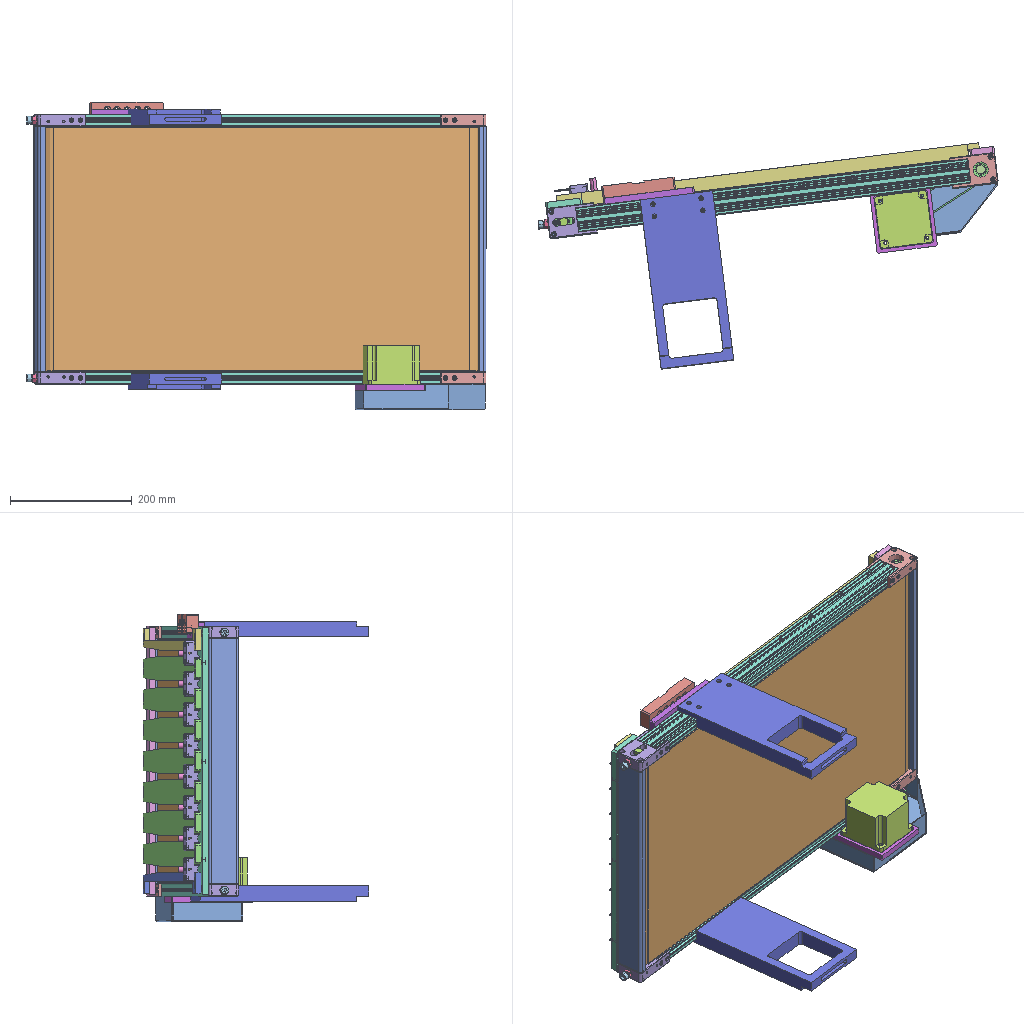Assembly | STEP file | 35 different items | 337 placed | box 756 x 372 x 506 mm
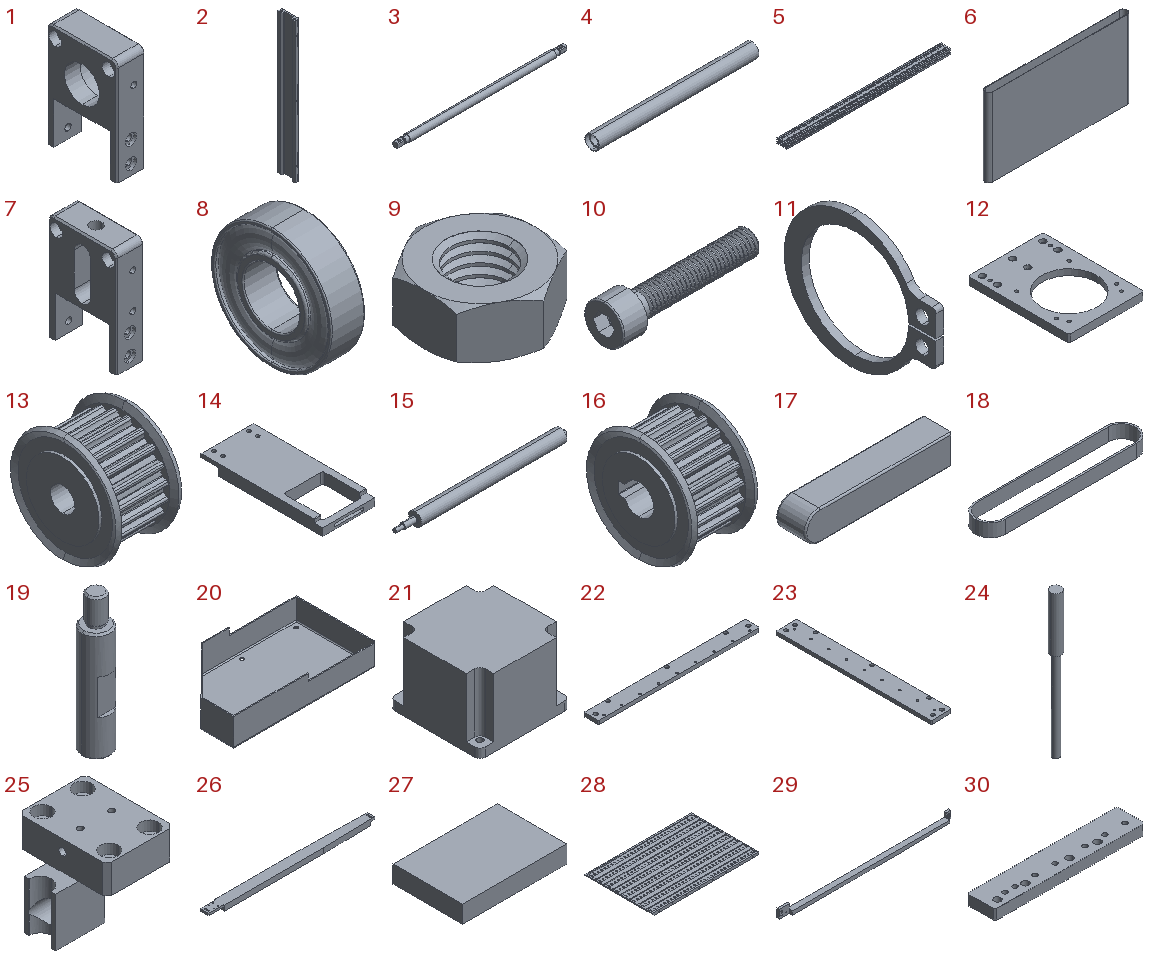Parts list (item | name | quantity | parent item | size | volume):
1 | PN_0002 | x2 | in 30 | 20 x 50 x 75 mm | 35811 mm3
2 | PN_0016 | x2 | in 30 | 12 x 50 x 404 mm | 142558 mm3
3 | PN_0017 | x1 | in 30 | 444 x 18 x 18 mm | 106069 mm3
4 | PN_0018 | x1 | in 30 | 402 x 36 x 36 mm | 206186 mm3
5 | PN_0005_default[machined] | x2 | in 30 | 650 x 40 x 20 mm | 192154 mm3
6 | PN_0019 | x1 | in 30 | 730 x 40 x 400 mm | 1199499 mm3
7 | PN_0011 | x2 | in 30 | 20 x 50 x 78 mm | 41890 mm3
8 | SUB6002ZZ_SUB6002ZZ | x4 | in 30 | 9 x 32 x 32 mm | 5285 mm3
9 | Hex nut M8 | x2 | in 30 | 13 x 15.011 x 6 mm | 626.264 mm3
10 | Socket head screw M8_L16 | x2 | in 30 | 48 x 13 x 13 mm | 2691 mm3
11 | STWN15_STWN15 | x2 | in 30 | 1 x 19.5 x 16.88 mm | 88.469 mm3
12 | PN_0008 | x1 | in 30 | 100 x 135 x 10 mm | 83048 mm3
13 | HTPA20S5M150-A-P9 | x1 | in 30 | 22 x 36 x 36 mm | 14035 mm3
14 | PN_0020 | x2 | in 30 | 120 x 280 x 25 mm | 533065 mm3
15 | PN_0015 | x1 | in 30 | 467 x 36 x 36 mm | 417063 mm3
16 | HTPA20S5M150-A-NK10 | x1 | in 30 | 22 x 36 x 36 mm | 13148 mm3
17 | KEG4-20 | x1 | in 30 | 20 x 4 x 4 mm | 312.344 mm3
18 | HTBN400S5M-150 | x1 | in 30 | 185.61 x 34.88 x 15 mm | 12143 mm3
19 | PN_0014 | x4 | in 30 | 8 x 8 x 39 mm | 1541 mm3
20 | PN_0009_default[machined] | x1 | in 30 | 210 x 118 x 42 mm | 64871 mm3
21 | 86HS35 | x1 | in 30 | 86 x 86 x 97 mm | 450020 mm3
22 | PN_0021 | x1 | in 30 | 444 x 40 x 10 mm | 172920 mm3
23 | PN_0007 | x1 | in 30 | 60 x 444 x 10 mm | 260719 mm3
24 | E3X-HD10+E32-ZD200E | x8 | in 30 | 3 x 3 x 40 mm | 169.646 mm3
25 | PN_0001 | x8 | in 30 | 40 x 40 x 35 mm | 19874 mm3
26 | PN_0003 | x7 | in 30 | 700 x 40.5 x 22 mm | 552490 mm3
27 | MISUMI magnet MGLF5-30-20 | x248 | in 30 | 30 x 20 x 5 mm | 3000 mm3
28 | PN_0012 | x1 | in 30 | 638 x 404 x 14 mm | 2739092 mm3
29 | PN_0013 | x1 | in 30 | 700 x 22 x 35 mm | 217020 mm3
30 | PN_0010 | x1 | in 30 | 150 x 28 x 10 mm | 38296 mm3
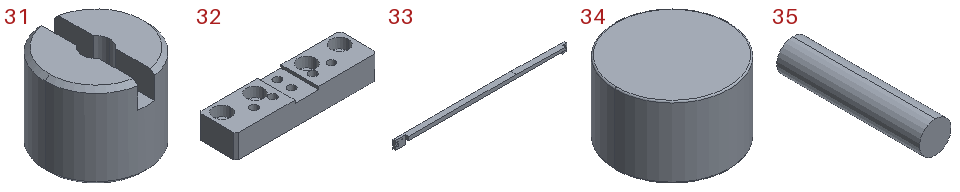31 | PN_0004 | x8 | in 30 | 12 x 12 x 10 mm | 792.649 mm3
32 | PN_0022 | x1 | in 30 | 120 x 32 x 20 mm | 59836 mm3
33 | PN_0006 | x1 | in 30 | 700 x 22 x 35 mm | 217020 mm3
34 | HXN8-5 | x8 | in 30 | 8 x 8 x 5 mm | 251.22 mm3
35 | 10440 | x8 | in 30 | 10 x 45 x 10 mm | 3534 mm3
Placements (level | parent | child | x y z in mm | rotation matrix by rows):
1 | 30 | PN_0002 | -446.325 52.298 -40.421 | 0 -0.124 0.9923 0 0.9923 0.124 -1 0 0
1 | 30 | PN_0002 | -446.325 52.298 -484.421 | 0 0.124 0.9923 0 -0.9923 0.124 1 0 -0
1 | 30 | PN_0016 | -421.022 55.461 -262.421 | 0.9923 0.124 0 0.124 -0.9923 0 0 0 -1
1 | 30 | PN_0016 | -1134.47 -33.72 -262.421 | -0.9923 0.124 0 -0.124 -0.9923 0 0 0 1
1 | 30 | PN_0017 | -1120.578 -31.984 -262.421 | 0 -0.124 -0.9923 0 0.9923 -0.124 1 0 -0
1 | 30 | PN_0018 | -1120.578 -31.984 -262.421 | 0 0.08753 -0.9962 0 0.9962 0.08753 1 0 0
1 | 30 | PN_0005_default[machined] | -545.305 39.925 -50.421 | 0.9923 -0.124 0 0.124 0.9923 0 0 0 1
1 | 30 | PN_0005_default[machined] | -545.305 39.925 -474.421 | 0.9923 -0.124 0 0.124 0.9923 0 0 0 1
1 | 30 | PN_0019 | -435.906 53.6 -262.421 | 0.9923 -0.124 0 0.124 0.9923 0 0 0 1
1 | 30 | PN_0011 | -1107.678 -30.371 -484.421 | 0 -0.124 -0.9923 0 0.9923 -0.124 1 0 -0
1 | 30 | PN_0011 | -1107.678 -30.371 -40.421 | 0 0.124 -0.9923 0 -0.9923 -0.124 -1 0 -0
1 | 30 | SUB6002ZZ_SUB6002ZZ | -1120.578 -31.984 -61.421 | 0 0.552 0.8339 0 0.8339 -0.552 -1 0 -0
1 | 30 | SUB6002ZZ_SUB6002ZZ | -1120.578 -31.984 -454.421 | 0 -0.6802 -0.733 0 -0.733 0.6802 -1 0 0
1 | 30 | SUB6002ZZ_SUB6002ZZ | -434.914 53.724 -51.421 | 0 -0.6117 -0.7911 0 -0.7911 0.6117 -1 0 0
1 | 30 | SUB6002ZZ_SUB6002ZZ | -434.914 53.724 -464.421 | 0 0.1138 0.9935 0 0.9935 -0.1138 -1 0 -0
1 | 30 | Hex nut M8 | -1146.377 -35.209 -474.421 | 0 -0.124 0.9923 0 0.9923 0.124 -1 0 0
1 | 30 | Hex nut M8 | -1146.377 -35.209 -50.421 | 0 -0.124 0.9923 0 0.9923 0.124 -1 0 0
1 | 30 | Socket head screw M8_L16 | -1162.254 -37.193 -474.421 | 0.9923 -0.1228 0.01771 0.124 0.9821 -0.1417 0 0.1428 0.9898
1 | 30 | Socket head screw M8_L16 | -1162.254 -37.193 -50.421 | 0.9923 -0.124 0 0.124 0.9923 0 0 0 1
1 | 30 | STWN15_STWN15 | -1120.578 -31.984 -463.921 | 0 0 1 0 1 0 -1 0 -0
1 | 30 | STWN15_STWN15 | -1120.578 -31.984 -60.921 | 0 0 1 0 1 0 -1 0 -0
1 | 30 | PN_0008 | -563.967 -10.277 -484.421 | -0.9923 -0.124 0 -0.124 0.9923 0 0 0 -1
1 | 30 | HTPA20S5M150-A-P9 | -561.796 -27.642 -518.521 | 0 0.4777 0.8785 0 -0.8785 0.4777 1 0 -0
1 | 30 | PN_0020 | -918.153 -127.615 -38.421 | 0.9923 -0.124 0 0.124 0.9923 0 0 0 1
1 | 30 | PN_0020 | -918.153 -127.615 -486.421 | -0.9923 -0.124 0 -0.124 0.9923 0 0 0 -1
1 | 30 | PN_0015 | -434.914 53.724 -518.521 | 0 -0.1715 -0.9852 0 0.9852 -0.1715 1 0 0
1 | 30 | HTPA20S5M150-A-NK10 | -434.914 53.724 -496.521 | 0 -0.1715 0.9852 0 0.9852 0.1715 -1 0 -0
1 | 30 | KEG4-20 | -435.686 58.158 -500.521 | 0 -0.1715 0.9852 0 0.9852 0.1715 -1 0 -0
1 | 30 | HTBN400S5M-150 | -517.393 0.8325 -500.021 | 0.8418 0.5398 0 0.5398 -0.8418 0 0 0 -1
1 | 30 | PN_0014 | -530.167 41.818 -509.921 | -0.3957 -0.9184 0 0.9184 -0.3957 0 0 0 1
1 | 30 | PN_0014 | -519.252 -45.503 -509.921 | -0.3957 -0.9184 0 0.9184 -0.3957 0 0 0 1
1 | 30 | PN_0014 | -598.634 -55.426 -509.921 | -0.3957 -0.9184 0 0.9184 -0.3957 0 0 0 1
1 | 30 | PN_0014 | -609.549 31.895 -509.921 | -0.3957 -0.9184 0 0.9184 -0.3957 0 0 0 1
1 | 30 | PN_0009_default[machined] | -510.446 4.979 -526.921 | -0.9923 0.124 0 -0.124 -0.9923 0 0 0 1
1 | 30 | 86HS35 | -561.796 -27.642 -486.421 | -0.9923 0.124 0 -0.124 -0.9923 0 0 0 1
1 | 30 | PN_0021 | -432.061 79.275 -262.421 | 0 0.9923 -0.124 0 0.124 0.9923 1 0 0
1 | 30 | PN_0007 | -1119.71 -6.681 -262.421 | -0.9923 0 -0.124 -0.124 0 0.9923 0 1 0
1 | 30 | E3X-HD10+E32-ZD200E | -1111.151 21.599 -440.221 | 0.0437 0.1161 0.9923 -0.3496 -0.9287 0.124 0.9359 -0.3523 -0
1 | 30 | PN_0001 | -1089.197 7.211 -440.221 | -0.9923 0 -0.124 -0.124 0 0.9923 0 1 0
1 | 30 | PN_0001 | -1089.197 7.211 -389.421 | -0.9923 0 -0.124 -0.124 0 0.9923 0 1 0
1 | 30 | PN_0001 | -1089.197 7.211 -338.621 | -0.9923 0 -0.124 -0.124 0 0.9923 0 1 0
1 | 30 | PN_0001 | -1089.197 7.211 -287.821 | -0.9923 0 -0.124 -0.124 0 0.9923 0 1 0
1 | 30 | PN_0001 | -1089.197 7.211 -237.021 | -0.9923 0 -0.124 -0.124 0 0.9923 0 1 0
1 | 30 | PN_0001 | -1089.197 7.211 -186.221 | -0.9923 0 -0.124 -0.124 0 0.9923 0 1 0
1 | 30 | PN_0001 | -1089.197 7.211 -135.421 | -0.9923 0 -0.124 -0.124 0 0.9923 0 1 0
1 | 30 | PN_0001 | -1089.197 7.211 -84.621 | -0.9923 0 -0.124 -0.124 0 0.9923 0 1 0
1 | 30 | E3X-HD10+E32-ZD200E | -1111.151 21.599 -389.421 | 0.0437 0.1161 0.9923 -0.3496 -0.9287 0.124 0.9359 -0.3523 -0
1 | 30 | E3X-HD10+E32-ZD200E | -1111.151 21.599 -338.621 | 0.0437 0.1161 0.9923 -0.3496 -0.9287 0.124 0.9359 -0.3523 -0
1 | 30 | E3X-HD10+E32-ZD200E | -1111.151 21.599 -287.821 | 0.0437 0.1161 0.9923 -0.3496 -0.9287 0.124 0.9359 -0.3523 -0
1 | 30 | E3X-HD10+E32-ZD200E | -1111.151 21.599 -237.021 | 0.0437 0.1161 0.9923 -0.3496 -0.9287 0.124 0.9359 -0.3523 -0
1 | 30 | E3X-HD10+E32-ZD200E | -1111.151 21.599 -186.221 | 0.0437 0.1161 0.9923 -0.3496 -0.9287 0.124 0.9359 -0.3523 -0
1 | 30 | E3X-HD10+E32-ZD200E | -1111.151 21.599 -135.421 | 0.0437 0.1161 0.9923 -0.3496 -0.9287 0.124 0.9359 -0.3523 -0
1 | 30 | E3X-HD10+E32-ZD200E | -1111.151 21.599 -84.621 | 0.0437 0.1161 0.9923 -0.3496 -0.9287 0.124 0.9359 -0.3523 -0
1 | 30 | PN_0003 | -782.856 32.403 -262.421 | 0.9923 0 -0.124 0.124 0 0.9923 0 -1 -0
1 | 30 | PN_0003 | -782.856 32.403 -414.821 | 0.9923 0 -0.124 0.124 0 0.9923 0 -1 -0
1 | 30 | MISUMI magnet MGLF5-30-20 | -1064.638 -11.89 -85.421 | 0 0.9923 -0.124 0 0.124 0.9923 1 0 0
1 | 30 | PN_0012 | -1082.375 -23.177 -60.421 | 0.9923 0 -0.124 0.124 0 0.9923 0 -1 -0
1 | 30 | PN_0013 | -785.027 49.768 -79.621 | 0.9923 -0.124 0 0.124 0.9923 0 0 0 1
1 | 30 | PN_0010 | -966.527 17.506 -46.421 | 0.9923 0 0.124 0.124 0 -0.9923 0 1 0
1 | 30 | PN_0004 | -1078.778 4.482 -84.621 | -0.123 -0.01626 -0.9923 0.9837 0.1301 -0.124 0.1311 -0.9914 0
1 | 30 | PN_0003 | -782.856 32.403 -110.021 | 0.9923 0 -0.124 0.124 0 0.9923 0 -1 -0
1 | 30 | PN_0003 | -782.856 32.403 -211.621 | 0.9923 0 -0.124 0.124 0 0.9923 0 -1 -0
1 | 30 | PN_0003 | -782.856 32.403 -160.821 | 0.9923 0 -0.124 0.124 0 0.9923 0 -1 -0
1 | 30 | PN_0003 | -782.856 32.403 -313.221 | 0.9923 0 -0.124 0.124 0 0.9923 0 -1 -0
1 | 30 | PN_0003 | -782.856 32.403 -364.021 | 0.9923 0 -0.124 0.124 0 0.9923 0 -1 -0
1 | 30 | PN_0022 | -1055.832 6.343 -20.421 | 0.9923 0 -0.124 0.124 0 0.9923 0 -1 -0
1 | 30 | PN_0004 | -1078.778 4.482 -135.421 | -0.123 -0.01626 -0.9923 0.9837 0.1301 -0.124 0.1311 -0.9914 0
1 | 30 | PN_0004 | -1078.778 4.482 -186.221 | -0.123 -0.01626 -0.9923 0.9837 0.1301 -0.124 0.1311 -0.9914 0
1 | 30 | PN_0004 | -1078.778 4.482 -237.021 | -0.123 -0.01626 -0.9923 0.9837 0.1301 -0.124 0.1311 -0.9914 0
1 | 30 | PN_0004 | -1078.778 4.482 -287.821 | -0.123 -0.01626 -0.9923 0.9837 0.1301 -0.124 0.1311 -0.9914 0
1 | 30 | PN_0004 | -1078.778 4.482 -338.621 | -0.123 -0.01626 -0.9923 0.9837 0.1301 -0.124 0.1311 -0.9914 0
1 | 30 | PN_0004 | -1078.778 4.482 -389.421 | -0.123 -0.01626 -0.9923 0.9837 0.1301 -0.124 0.1311 -0.9914 0
1 | 30 | PN_0004 | -1078.778 4.482 -440.221 | -0.123 -0.01626 -0.9923 0.9837 0.1301 -0.124 0.1311 -0.9914 0
1 | 30 | MISUMI magnet MGLF5-30-20 | -1064.638 -11.89 -136.221 | 0 0.9923 -0.124 0 0.124 0.9923 1 0 0
1 | 30 | MISUMI magnet MGLF5-30-20 | -1064.638 -11.89 -187.021 | 0 0.9923 -0.124 0 0.124 0.9923 1 0 0
1 | 30 | MISUMI magnet MGLF5-30-20 | -1064.638 -11.89 -237.821 | 0 0.9923 -0.124 0 0.124 0.9923 1 0 0
1 | 30 | MISUMI magnet MGLF5-30-20 | -1064.638 -11.89 -288.621 | 0 0.9923 -0.124 0 0.124 0.9923 1 0 0
1 | 30 | MISUMI magnet MGLF5-30-20 | -1064.638 -11.89 -339.421 | 0 0.9923 -0.124 0 0.124 0.9923 1 0 0
1 | 30 | MISUMI magnet MGLF5-30-20 | -1064.638 -11.89 -390.221 | 0 0.9923 -0.124 0 0.124 0.9923 1 0 0
1 | 30 | MISUMI magnet MGLF5-30-20 | -1064.638 -11.89 -441.021 | 0 0.9923 -0.124 0 0.124 0.9923 1 0 0
1 | 30 | MISUMI magnet MGLF5-30-20 | -1044.793 -9.409 -85.421 | 0 0.9923 -0.124 0 0.124 0.9923 1 0 0
1 | 30 | MISUMI magnet MGLF5-30-20 | -1044.793 -9.409 -136.221 | 0 0.9923 -0.124 0 0.124 0.9923 1 0 0
1 | 30 | MISUMI magnet MGLF5-30-20 | -1044.793 -9.409 -187.021 | 0 0.9923 -0.124 0 0.124 0.9923 1 0 0
1 | 30 | MISUMI magnet MGLF5-30-20 | -1044.793 -9.409 -237.821 | 0 0.9923 -0.124 0 0.124 0.9923 1 0 0
1 | 30 | MISUMI magnet MGLF5-30-20 | -1044.793 -9.409 -288.621 | 0 0.9923 -0.124 0 0.124 0.9923 1 0 0
1 | 30 | MISUMI magnet MGLF5-30-20 | -1044.793 -9.409 -339.421 | 0 0.9923 -0.124 0 0.124 0.9923 1 0 0
1 | 30 | MISUMI magnet MGLF5-30-20 | -1044.793 -9.409 -390.221 | 0 0.9923 -0.124 0 0.124 0.9923 1 0 0
1 | 30 | MISUMI magnet MGLF5-30-20 | -1044.793 -9.409 -441.021 | 0 0.9923 -0.124 0 0.124 0.9923 1 0 0
1 | 30 | MISUMI magnet MGLF5-30-20 | -1024.947 -6.929 -85.421 | 0 0.9923 -0.124 0 0.124 0.9923 1 0 0
1 | 30 | MISUMI magnet MGLF5-30-20 | -1024.947 -6.929 -136.221 | 0 0.9923 -0.124 0 0.124 0.9923 1 0 0
1 | 30 | MISUMI magnet MGLF5-30-20 | -1024.947 -6.929 -187.021 | 0 0.9923 -0.124 0 0.124 0.9923 1 0 0
1 | 30 | MISUMI magnet MGLF5-30-20 | -1024.947 -6.929 -237.821 | 0 0.9923 -0.124 0 0.124 0.9923 1 0 0
1 | 30 | MISUMI magnet MGLF5-30-20 | -1024.947 -6.929 -288.621 | 0 0.9923 -0.124 0 0.124 0.9923 1 0 0
1 | 30 | MISUMI magnet MGLF5-30-20 | -1024.947 -6.929 -339.421 | 0 0.9923 -0.124 0 0.124 0.9923 1 0 0
1 | 30 | MISUMI magnet MGLF5-30-20 | -1024.947 -6.929 -390.221 | 0 0.9923 -0.124 0 0.124 0.9923 1 0 0
1 | 30 | MISUMI magnet MGLF5-30-20 | -1024.947 -6.929 -441.021 | 0 0.9923 -0.124 0 0.124 0.9923 1 0 0
1 | 30 | MISUMI magnet MGLF5-30-20 | -1005.102 -4.448 -85.421 | 0 0.9923 -0.124 0 0.124 0.9923 1 0 0
1 | 30 | MISUMI magnet MGLF5-30-20 | -1005.102 -4.448 -136.221 | 0 0.9923 -0.124 0 0.124 0.9923 1 0 0
1 | 30 | MISUMI magnet MGLF5-30-20 | -1005.102 -4.448 -187.021 | 0 0.9923 -0.124 0 0.124 0.9923 1 0 0
1 | 30 | MISUMI magnet MGLF5-30-20 | -1005.102 -4.448 -237.821 | 0 0.9923 -0.124 0 0.124 0.9923 1 0 0
1 | 30 | MISUMI magnet MGLF5-30-20 | -1005.102 -4.448 -288.621 | 0 0.9923 -0.124 0 0.124 0.9923 1 0 0
1 | 30 | MISUMI magnet MGLF5-30-20 | -1005.102 -4.448 -339.421 | 0 0.9923 -0.124 0 0.124 0.9923 1 0 0
1 | 30 | MISUMI magnet MGLF5-30-20 | -1005.102 -4.448 -390.221 | 0 0.9923 -0.124 0 0.124 0.9923 1 0 0
1 | 30 | MISUMI magnet MGLF5-30-20 | -1005.102 -4.448 -441.021 | 0 0.9923 -0.124 0 0.124 0.9923 1 0 0
1 | 30 | MISUMI magnet MGLF5-30-20 | -985.256 -1.967 -85.421 | 0 0.9923 -0.124 0 0.124 0.9923 1 0 0
1 | 30 | MISUMI magnet MGLF5-30-20 | -985.256 -1.967 -136.221 | 0 0.9923 -0.124 0 0.124 0.9923 1 0 0
1 | 30 | MISUMI magnet MGLF5-30-20 | -985.256 -1.967 -187.021 | 0 0.9923 -0.124 0 0.124 0.9923 1 0 0
1 | 30 | MISUMI magnet MGLF5-30-20 | -985.256 -1.967 -237.821 | 0 0.9923 -0.124 0 0.124 0.9923 1 0 0
1 | 30 | MISUMI magnet MGLF5-30-20 | -985.256 -1.967 -288.621 | 0 0.9923 -0.124 0 0.124 0.9923 1 0 0
1 | 30 | MISUMI magnet MGLF5-30-20 | -985.256 -1.967 -339.421 | 0 0.9923 -0.124 0 0.124 0.9923 1 0 0
1 | 30 | MISUMI magnet MGLF5-30-20 | -985.256 -1.967 -390.221 | 0 0.9923 -0.124 0 0.124 0.9923 1 0 0
1 | 30 | MISUMI magnet MGLF5-30-20 | -985.256 -1.967 -441.021 | 0 0.9923 -0.124 0 0.124 0.9923 1 0 0
1 | 30 | MISUMI magnet MGLF5-30-20 | -965.41 0.5134 -85.421 | 0 0.9923 -0.124 0 0.124 0.9923 1 0 0
1 | 30 | MISUMI magnet MGLF5-30-20 | -965.41 0.5134 -136.221 | 0 0.9923 -0.124 0 0.124 0.9923 1 0 0
1 | 30 | MISUMI magnet MGLF5-30-20 | -965.41 0.5134 -187.021 | 0 0.9923 -0.124 0 0.124 0.9923 1 0 0
1 | 30 | MISUMI magnet MGLF5-30-20 | -965.41 0.5134 -237.821 | 0 0.9923 -0.124 0 0.124 0.9923 1 0 0
1 | 30 | MISUMI magnet MGLF5-30-20 | -965.41 0.5134 -288.621 | 0 0.9923 -0.124 0 0.124 0.9923 1 0 0
1 | 30 | MISUMI magnet MGLF5-30-20 | -965.41 0.5134 -339.421 | 0 0.9923 -0.124 0 0.124 0.9923 1 0 0
1 | 30 | MISUMI magnet MGLF5-30-20 | -965.41 0.5134 -390.221 | 0 0.9923 -0.124 0 0.124 0.9923 1 0 0
1 | 30 | MISUMI magnet MGLF5-30-20 | -965.41 0.5134 -441.021 | 0 0.9923 -0.124 0 0.124 0.9923 1 0 0
1 | 30 | MISUMI magnet MGLF5-30-20 | -945.565 2.994 -85.421 | 0 0.9923 -0.124 0 0.124 0.9923 1 0 0
1 | 30 | MISUMI magnet MGLF5-30-20 | -945.565 2.994 -136.221 | 0 0.9923 -0.124 0 0.124 0.9923 1 0 0
1 | 30 | MISUMI magnet MGLF5-30-20 | -945.565 2.994 -187.021 | 0 0.9923 -0.124 0 0.124 0.9923 1 0 0
1 | 30 | MISUMI magnet MGLF5-30-20 | -945.565 2.994 -237.821 | 0 0.9923 -0.124 0 0.124 0.9923 1 0 0
1 | 30 | MISUMI magnet MGLF5-30-20 | -945.565 2.994 -288.621 | 0 0.9923 -0.124 0 0.124 0.9923 1 0 0
1 | 30 | MISUMI magnet MGLF5-30-20 | -945.565 2.994 -339.421 | 0 0.9923 -0.124 0 0.124 0.9923 1 0 0
1 | 30 | MISUMI magnet MGLF5-30-20 | -945.565 2.994 -390.221 | 0 0.9923 -0.124 0 0.124 0.9923 1 0 0
1 | 30 | MISUMI magnet MGLF5-30-20 | -945.565 2.994 -441.021 | 0 0.9923 -0.124 0 0.124 0.9923 1 0 0
1 | 30 | MISUMI magnet MGLF5-30-20 | -925.719 5.475 -85.421 | 0 0.9923 -0.124 0 0.124 0.9923 1 0 0
1 | 30 | MISUMI magnet MGLF5-30-20 | -925.719 5.475 -136.221 | 0 0.9923 -0.124 0 0.124 0.9923 1 0 0
1 | 30 | MISUMI magnet MGLF5-30-20 | -925.719 5.475 -187.021 | 0 0.9923 -0.124 0 0.124 0.9923 1 0 0
1 | 30 | MISUMI magnet MGLF5-30-20 | -925.719 5.475 -237.821 | 0 0.9923 -0.124 0 0.124 0.9923 1 0 0
1 | 30 | MISUMI magnet MGLF5-30-20 | -925.719 5.475 -288.621 | 0 0.9923 -0.124 0 0.124 0.9923 1 0 0
1 | 30 | MISUMI magnet MGLF5-30-20 | -925.719 5.475 -339.421 | 0 0.9923 -0.124 0 0.124 0.9923 1 0 0
1 | 30 | MISUMI magnet MGLF5-30-20 | -925.719 5.475 -390.221 | 0 0.9923 -0.124 0 0.124 0.9923 1 0 0
1 | 30 | MISUMI magnet MGLF5-30-20 | -925.719 5.475 -441.021 | 0 0.9923 -0.124 0 0.124 0.9923 1 0 0
1 | 30 | MISUMI magnet MGLF5-30-20 | -905.874 7.955 -85.421 | 0 0.9923 -0.124 0 0.124 0.9923 1 0 0
1 | 30 | MISUMI magnet MGLF5-30-20 | -905.874 7.955 -136.221 | 0 0.9923 -0.124 0 0.124 0.9923 1 0 0
1 | 30 | MISUMI magnet MGLF5-30-20 | -905.874 7.955 -187.021 | 0 0.9923 -0.124 0 0.124 0.9923 1 0 0
1 | 30 | MISUMI magnet MGLF5-30-20 | -905.874 7.955 -237.821 | 0 0.9923 -0.124 0 0.124 0.9923 1 0 0
1 | 30 | MISUMI magnet MGLF5-30-20 | -905.874 7.955 -288.621 | 0 0.9923 -0.124 0 0.124 0.9923 1 0 0
1 | 30 | MISUMI magnet MGLF5-30-20 | -905.874 7.955 -339.421 | 0 0.9923 -0.124 0 0.124 0.9923 1 0 0
1 | 30 | MISUMI magnet MGLF5-30-20 | -905.874 7.955 -390.221 | 0 0.9923 -0.124 0 0.124 0.9923 1 0 0
1 | 30 | MISUMI magnet MGLF5-30-20 | -905.874 7.955 -441.021 | 0 0.9923 -0.124 0 0.124 0.9923 1 0 0
1 | 30 | MISUMI magnet MGLF5-30-20 | -886.028 10.436 -85.421 | 0 0.9923 -0.124 0 0.124 0.9923 1 0 0
1 | 30 | MISUMI magnet MGLF5-30-20 | -886.028 10.436 -136.221 | 0 0.9923 -0.124 0 0.124 0.9923 1 0 0
1 | 30 | MISUMI magnet MGLF5-30-20 | -886.028 10.436 -187.021 | 0 0.9923 -0.124 0 0.124 0.9923 1 0 0
1 | 30 | MISUMI magnet MGLF5-30-20 | -886.028 10.436 -237.821 | 0 0.9923 -0.124 0 0.124 0.9923 1 0 0
1 | 30 | MISUMI magnet MGLF5-30-20 | -886.028 10.436 -288.621 | 0 0.9923 -0.124 0 0.124 0.9923 1 0 0
1 | 30 | MISUMI magnet MGLF5-30-20 | -886.028 10.436 -339.421 | 0 0.9923 -0.124 0 0.124 0.9923 1 0 0
1 | 30 | MISUMI magnet MGLF5-30-20 | -886.028 10.436 -390.221 | 0 0.9923 -0.124 0 0.124 0.9923 1 0 0
1 | 30 | MISUMI magnet MGLF5-30-20 | -886.028 10.436 -441.021 | 0 0.9923 -0.124 0 0.124 0.9923 1 0 0
1 | 30 | MISUMI magnet MGLF5-30-20 | -866.183 12.917 -85.421 | 0 0.9923 -0.124 0 0.124 0.9923 1 0 0
1 | 30 | MISUMI magnet MGLF5-30-20 | -866.183 12.917 -136.221 | 0 0.9923 -0.124 0 0.124 0.9923 1 0 0
1 | 30 | MISUMI magnet MGLF5-30-20 | -866.183 12.917 -187.021 | 0 0.9923 -0.124 0 0.124 0.9923 1 0 0
1 | 30 | MISUMI magnet MGLF5-30-20 | -866.183 12.917 -237.821 | 0 0.9923 -0.124 0 0.124 0.9923 1 0 0
1 | 30 | MISUMI magnet MGLF5-30-20 | -866.183 12.917 -288.621 | 0 0.9923 -0.124 0 0.124 0.9923 1 0 0
1 | 30 | MISUMI magnet MGLF5-30-20 | -866.183 12.917 -339.421 | 0 0.9923 -0.124 0 0.124 0.9923 1 0 0
1 | 30 | MISUMI magnet MGLF5-30-20 | -866.183 12.917 -390.221 | 0 0.9923 -0.124 0 0.124 0.9923 1 0 0
1 | 30 | MISUMI magnet MGLF5-30-20 | -866.183 12.917 -441.021 | 0 0.9923 -0.124 0 0.124 0.9923 1 0 0
1 | 30 | MISUMI magnet MGLF5-30-20 | -846.337 15.398 -85.421 | 0 0.9923 -0.124 0 0.124 0.9923 1 0 0
1 | 30 | MISUMI magnet MGLF5-30-20 | -846.337 15.398 -136.221 | 0 0.9923 -0.124 0 0.124 0.9923 1 0 0
1 | 30 | MISUMI magnet MGLF5-30-20 | -846.337 15.398 -187.021 | 0 0.9923 -0.124 0 0.124 0.9923 1 0 0
1 | 30 | MISUMI magnet MGLF5-30-20 | -846.337 15.398 -237.821 | 0 0.9923 -0.124 0 0.124 0.9923 1 0 0
1 | 30 | MISUMI magnet MGLF5-30-20 | -846.337 15.398 -288.621 | 0 0.9923 -0.124 0 0.124 0.9923 1 0 0
1 | 30 | MISUMI magnet MGLF5-30-20 | -846.337 15.398 -339.421 | 0 0.9923 -0.124 0 0.124 0.9923 1 0 0
1 | 30 | MISUMI magnet MGLF5-30-20 | -846.337 15.398 -390.221 | 0 0.9923 -0.124 0 0.124 0.9923 1 0 0
1 | 30 | MISUMI magnet MGLF5-30-20 | -846.337 15.398 -441.021 | 0 0.9923 -0.124 0 0.124 0.9923 1 0 0
1 | 30 | MISUMI magnet MGLF5-30-20 | -826.492 17.878 -85.421 | 0 0.9923 -0.124 0 0.124 0.9923 1 0 0
1 | 30 | MISUMI magnet MGLF5-30-20 | -826.492 17.878 -136.221 | 0 0.9923 -0.124 0 0.124 0.9923 1 0 0
1 | 30 | MISUMI magnet MGLF5-30-20 | -826.492 17.878 -187.021 | 0 0.9923 -0.124 0 0.124 0.9923 1 0 0
1 | 30 | MISUMI magnet MGLF5-30-20 | -826.492 17.878 -237.821 | 0 0.9923 -0.124 0 0.124 0.9923 1 0 0
1 | 30 | MISUMI magnet MGLF5-30-20 | -826.492 17.878 -288.621 | 0 0.9923 -0.124 0 0.124 0.9923 1 0 0
1 | 30 | MISUMI magnet MGLF5-30-20 | -826.492 17.878 -339.421 | 0 0.9923 -0.124 0 0.124 0.9923 1 0 0
1 | 30 | MISUMI magnet MGLF5-30-20 | -826.492 17.878 -390.221 | 0 0.9923 -0.124 0 0.124 0.9923 1 0 0
1 | 30 | MISUMI magnet MGLF5-30-20 | -826.492 17.878 -441.021 | 0 0.9923 -0.124 0 0.124 0.9923 1 0 0
1 | 30 | MISUMI magnet MGLF5-30-20 | -806.646 20.359 -85.421 | 0 0.9923 -0.124 0 0.124 0.9923 1 0 0
1 | 30 | MISUMI magnet MGLF5-30-20 | -806.646 20.359 -136.221 | 0 0.9923 -0.124 0 0.124 0.9923 1 0 0
1 | 30 | MISUMI magnet MGLF5-30-20 | -806.646 20.359 -187.021 | 0 0.9923 -0.124 0 0.124 0.9923 1 0 0
1 | 30 | MISUMI magnet MGLF5-30-20 | -806.646 20.359 -237.821 | 0 0.9923 -0.124 0 0.124 0.9923 1 0 0
1 | 30 | MISUMI magnet MGLF5-30-20 | -806.646 20.359 -288.621 | 0 0.9923 -0.124 0 0.124 0.9923 1 0 0
1 | 30 | MISUMI magnet MGLF5-30-20 | -806.646 20.359 -339.421 | 0 0.9923 -0.124 0 0.124 0.9923 1 0 0
1 | 30 | MISUMI magnet MGLF5-30-20 | -806.646 20.359 -390.221 | 0 0.9923 -0.124 0 0.124 0.9923 1 0 0
1 | 30 | MISUMI magnet MGLF5-30-20 | -806.646 20.359 -441.021 | 0 0.9923 -0.124 0 0.124 0.9923 1 0 0
1 | 30 | MISUMI magnet MGLF5-30-20 | -786.801 22.84 -85.421 | 0 0.9923 -0.124 0 0.124 0.9923 1 0 0
1 | 30 | MISUMI magnet MGLF5-30-20 | -786.801 22.84 -136.221 | 0 0.9923 -0.124 0 0.124 0.9923 1 0 0
1 | 30 | MISUMI magnet MGLF5-30-20 | -786.801 22.84 -187.021 | 0 0.9923 -0.124 0 0.124 0.9923 1 0 0
1 | 30 | MISUMI magnet MGLF5-30-20 | -786.801 22.84 -237.821 | 0 0.9923 -0.124 0 0.124 0.9923 1 0 0
1 | 30 | MISUMI magnet MGLF5-30-20 | -786.801 22.84 -288.621 | 0 0.9923 -0.124 0 0.124 0.9923 1 0 0
1 | 30 | MISUMI magnet MGLF5-30-20 | -786.801 22.84 -339.421 | 0 0.9923 -0.124 0 0.124 0.9923 1 0 0
1 | 30 | MISUMI magnet MGLF5-30-20 | -786.801 22.84 -390.221 | 0 0.9923 -0.124 0 0.124 0.9923 1 0 0
1 | 30 | MISUMI magnet MGLF5-30-20 | -786.801 22.84 -441.021 | 0 0.9923 -0.124 0 0.124 0.9923 1 0 0
1 | 30 | MISUMI magnet MGLF5-30-20 | -766.955 25.32 -85.421 | 0 0.9923 -0.124 0 0.124 0.9923 1 0 0
1 | 30 | MISUMI magnet MGLF5-30-20 | -766.955 25.32 -136.221 | 0 0.9923 -0.124 0 0.124 0.9923 1 0 0
1 | 30 | MISUMI magnet MGLF5-30-20 | -766.955 25.32 -187.021 | 0 0.9923 -0.124 0 0.124 0.9923 1 0 0
1 | 30 | MISUMI magnet MGLF5-30-20 | -766.955 25.32 -237.821 | 0 0.9923 -0.124 0 0.124 0.9923 1 0 0
1 | 30 | MISUMI magnet MGLF5-30-20 | -766.955 25.32 -288.621 | 0 0.9923 -0.124 0 0.124 0.9923 1 0 0
1 | 30 | MISUMI magnet MGLF5-30-20 | -766.955 25.32 -339.421 | 0 0.9923 -0.124 0 0.124 0.9923 1 0 0
1 | 30 | MISUMI magnet MGLF5-30-20 | -766.955 25.32 -390.221 | 0 0.9923 -0.124 0 0.124 0.9923 1 0 0
1 | 30 | MISUMI magnet MGLF5-30-20 | -766.955 25.32 -441.021 | 0 0.9923 -0.124 0 0.124 0.9923 1 0 0
1 | 30 | MISUMI magnet MGLF5-30-20 | -747.109 27.801 -85.421 | 0 0.9923 -0.124 0 0.124 0.9923 1 0 0
1 | 30 | MISUMI magnet MGLF5-30-20 | -747.109 27.801 -136.221 | 0 0.9923 -0.124 0 0.124 0.9923 1 0 0
1 | 30 | MISUMI magnet MGLF5-30-20 | -747.109 27.801 -187.021 | 0 0.9923 -0.124 0 0.124 0.9923 1 0 0
1 | 30 | MISUMI magnet MGLF5-30-20 | -747.109 27.801 -237.821 | 0 0.9923 -0.124 0 0.124 0.9923 1 0 0
1 | 30 | MISUMI magnet MGLF5-30-20 | -747.109 27.801 -288.621 | 0 0.9923 -0.124 0 0.124 0.9923 1 0 0
1 | 30 | MISUMI magnet MGLF5-30-20 | -747.109 27.801 -339.421 | 0 0.9923 -0.124 0 0.124 0.9923 1 0 0
1 | 30 | MISUMI magnet MGLF5-30-20 | -747.109 27.801 -390.221 | 0 0.9923 -0.124 0 0.124 0.9923 1 0 0
1 | 30 | MISUMI magnet MGLF5-30-20 | -747.109 27.801 -441.021 | 0 0.9923 -0.124 0 0.124 0.9923 1 0 0
1 | 30 | MISUMI magnet MGLF5-30-20 | -727.264 30.282 -85.421 | 0 0.9923 -0.124 0 0.124 0.9923 1 0 0
1 | 30 | MISUMI magnet MGLF5-30-20 | -727.264 30.282 -136.221 | 0 0.9923 -0.124 0 0.124 0.9923 1 0 0
1 | 30 | MISUMI magnet MGLF5-30-20 | -727.264 30.282 -187.021 | 0 0.9923 -0.124 0 0.124 0.9923 1 0 0
1 | 30 | MISUMI magnet MGLF5-30-20 | -727.264 30.282 -237.821 | 0 0.9923 -0.124 0 0.124 0.9923 1 0 0
1 | 30 | MISUMI magnet MGLF5-30-20 | -727.264 30.282 -288.621 | 0 0.9923 -0.124 0 0.124 0.9923 1 0 0
1 | 30 | MISUMI magnet MGLF5-30-20 | -727.264 30.282 -339.421 | 0 0.9923 -0.124 0 0.124 0.9923 1 0 0
1 | 30 | MISUMI magnet MGLF5-30-20 | -727.264 30.282 -390.221 | 0 0.9923 -0.124 0 0.124 0.9923 1 0 0
1 | 30 | MISUMI magnet MGLF5-30-20 | -727.264 30.282 -441.021 | 0 0.9923 -0.124 0 0.124 0.9923 1 0 0
1 | 30 | MISUMI magnet MGLF5-30-20 | -707.418 32.762 -85.421 | 0 0.9923 -0.124 0 0.124 0.9923 1 0 0
1 | 30 | MISUMI magnet MGLF5-30-20 | -707.418 32.762 -136.221 | 0 0.9923 -0.124 0 0.124 0.9923 1 0 0
1 | 30 | MISUMI magnet MGLF5-30-20 | -707.418 32.762 -187.021 | 0 0.9923 -0.124 0 0.124 0.9923 1 0 0
1 | 30 | MISUMI magnet MGLF5-30-20 | -707.418 32.762 -237.821 | 0 0.9923 -0.124 0 0.124 0.9923 1 0 0
1 | 30 | MISUMI magnet MGLF5-30-20 | -707.418 32.762 -288.621 | 0 0.9923 -0.124 0 0.124 0.9923 1 0 0
1 | 30 | MISUMI magnet MGLF5-30-20 | -707.418 32.762 -339.421 | 0 0.9923 -0.124 0 0.124 0.9923 1 0 0
1 | 30 | MISUMI magnet MGLF5-30-20 | -707.418 32.762 -390.221 | 0 0.9923 -0.124 0 0.124 0.9923 1 0 0
1 | 30 | MISUMI magnet MGLF5-30-20 | -707.418 32.762 -441.021 | 0 0.9923 -0.124 0 0.124 0.9923 1 0 0
1 | 30 | MISUMI magnet MGLF5-30-20 | -687.573 35.243 -85.421 | 0 0.9923 -0.124 0 0.124 0.9923 1 0 0
1 | 30 | MISUMI magnet MGLF5-30-20 | -687.573 35.243 -136.221 | 0 0.9923 -0.124 0 0.124 0.9923 1 0 0
1 | 30 | MISUMI magnet MGLF5-30-20 | -687.573 35.243 -187.021 | 0 0.9923 -0.124 0 0.124 0.9923 1 0 0
1 | 30 | MISUMI magnet MGLF5-30-20 | -687.573 35.243 -237.821 | 0 0.9923 -0.124 0 0.124 0.9923 1 0 0
1 | 30 | MISUMI magnet MGLF5-30-20 | -687.573 35.243 -288.621 | 0 0.9923 -0.124 0 0.124 0.9923 1 0 0
1 | 30 | MISUMI magnet MGLF5-30-20 | -687.573 35.243 -339.421 | 0 0.9923 -0.124 0 0.124 0.9923 1 0 0
1 | 30 | MISUMI magnet MGLF5-30-20 | -687.573 35.243 -390.221 | 0 0.9923 -0.124 0 0.124 0.9923 1 0 0
1 | 30 | MISUMI magnet MGLF5-30-20 | -687.573 35.243 -441.021 | 0 0.9923 -0.124 0 0.124 0.9923 1 0 0
1 | 30 | MISUMI magnet MGLF5-30-20 | -667.727 37.724 -85.421 | 0 0.9923 -0.124 0 0.124 0.9923 1 0 0
1 | 30 | MISUMI magnet MGLF5-30-20 | -667.727 37.724 -136.221 | 0 0.9923 -0.124 0 0.124 0.9923 1 0 0
1 | 30 | MISUMI magnet MGLF5-30-20 | -667.727 37.724 -187.021 | 0 0.9923 -0.124 0 0.124 0.9923 1 0 0
1 | 30 | MISUMI magnet MGLF5-30-20 | -667.727 37.724 -237.821 | 0 0.9923 -0.124 0 0.124 0.9923 1 0 0
1 | 30 | MISUMI magnet MGLF5-30-20 | -667.727 37.724 -288.621 | 0 0.9923 -0.124 0 0.124 0.9923 1 0 0
1 | 30 | MISUMI magnet MGLF5-30-20 | -667.727 37.724 -339.421 | 0 0.9923 -0.124 0 0.124 0.9923 1 0 0
1 | 30 | MISUMI magnet MGLF5-30-20 | -667.727 37.724 -390.221 | 0 0.9923 -0.124 0 0.124 0.9923 1 0 0
1 | 30 | MISUMI magnet MGLF5-30-20 | -667.727 37.724 -441.021 | 0 0.9923 -0.124 0 0.124 0.9923 1 0 0
1 | 30 | MISUMI magnet MGLF5-30-20 | -647.882 40.205 -85.421 | 0 0.9923 -0.124 0 0.124 0.9923 1 0 0
1 | 30 | MISUMI magnet MGLF5-30-20 | -647.882 40.205 -136.221 | 0 0.9923 -0.124 0 0.124 0.9923 1 0 0
1 | 30 | MISUMI magnet MGLF5-30-20 | -647.882 40.205 -187.021 | 0 0.9923 -0.124 0 0.124 0.9923 1 0 0
1 | 30 | MISUMI magnet MGLF5-30-20 | -647.882 40.205 -237.821 | 0 0.9923 -0.124 0 0.124 0.9923 1 0 0
1 | 30 | MISUMI magnet MGLF5-30-20 | -647.882 40.205 -288.621 | 0 0.9923 -0.124 0 0.124 0.9923 1 0 0
1 | 30 | MISUMI magnet MGLF5-30-20 | -647.882 40.205 -339.421 | 0 0.9923 -0.124 0 0.124 0.9923 1 0 0
1 | 30 | MISUMI magnet MGLF5-30-20 | -647.882 40.205 -390.221 | 0 0.9923 -0.124 0 0.124 0.9923 1 0 0
1 | 30 | MISUMI magnet MGLF5-30-20 | -647.882 40.205 -441.021 | 0 0.9923 -0.124 0 0.124 0.9923 1 0 0
1 | 30 | MISUMI magnet MGLF5-30-20 | -628.036 42.685 -85.421 | 0 0.9923 -0.124 0 0.124 0.9923 1 0 0
1 | 30 | MISUMI magnet MGLF5-30-20 | -628.036 42.685 -136.221 | 0 0.9923 -0.124 0 0.124 0.9923 1 0 0
1 | 30 | MISUMI magnet MGLF5-30-20 | -628.036 42.685 -187.021 | 0 0.9923 -0.124 0 0.124 0.9923 1 0 0
1 | 30 | MISUMI magnet MGLF5-30-20 | -628.036 42.685 -237.821 | 0 0.9923 -0.124 0 0.124 0.9923 1 0 0
1 | 30 | MISUMI magnet MGLF5-30-20 | -628.036 42.685 -288.621 | 0 0.9923 -0.124 0 0.124 0.9923 1 0 0
1 | 30 | MISUMI magnet MGLF5-30-20 | -628.036 42.685 -339.421 | 0 0.9923 -0.124 0 0.124 0.9923 1 0 0
1 | 30 | MISUMI magnet MGLF5-30-20 | -628.036 42.685 -390.221 | 0 0.9923 -0.124 0 0.124 0.9923 1 0 0
1 | 30 | MISUMI magnet MGLF5-30-20 | -628.036 42.685 -441.021 | 0 0.9923 -0.124 0 0.124 0.9923 1 0 0
1 | 30 | MISUMI magnet MGLF5-30-20 | -608.19 45.166 -85.421 | 0 0.9923 -0.124 0 0.124 0.9923 1 0 0
1 | 30 | MISUMI magnet MGLF5-30-20 | -608.19 45.166 -136.221 | 0 0.9923 -0.124 0 0.124 0.9923 1 0 0
1 | 30 | MISUMI magnet MGLF5-30-20 | -608.19 45.166 -187.021 | 0 0.9923 -0.124 0 0.124 0.9923 1 0 0
1 | 30 | MISUMI magnet MGLF5-30-20 | -608.19 45.166 -237.821 | 0 0.9923 -0.124 0 0.124 0.9923 1 0 0
1 | 30 | MISUMI magnet MGLF5-30-20 | -608.19 45.166 -288.621 | 0 0.9923 -0.124 0 0.124 0.9923 1 0 0
1 | 30 | MISUMI magnet MGLF5-30-20 | -608.19 45.166 -339.421 | 0 0.9923 -0.124 0 0.124 0.9923 1 0 0
1 | 30 | MISUMI magnet MGLF5-30-20 | -608.19 45.166 -390.221 | 0 0.9923 -0.124 0 0.124 0.9923 1 0 0
1 | 30 | MISUMI magnet MGLF5-30-20 | -608.19 45.166 -441.021 | 0 0.9923 -0.124 0 0.124 0.9923 1 0 0
1 | 30 | MISUMI magnet MGLF5-30-20 | -588.345 47.647 -85.421 | 0 0.9923 -0.124 0 0.124 0.9923 1 0 0
1 | 30 | MISUMI magnet MGLF5-30-20 | -588.345 47.647 -136.221 | 0 0.9923 -0.124 0 0.124 0.9923 1 0 0
1 | 30 | MISUMI magnet MGLF5-30-20 | -588.345 47.647 -187.021 | 0 0.9923 -0.124 0 0.124 0.9923 1 0 0
1 | 30 | MISUMI magnet MGLF5-30-20 | -588.345 47.647 -237.821 | 0 0.9923 -0.124 0 0.124 0.9923 1 0 0
1 | 30 | MISUMI magnet MGLF5-30-20 | -588.345 47.647 -288.621 | 0 0.9923 -0.124 0 0.124 0.9923 1 0 0
1 | 30 | MISUMI magnet MGLF5-30-20 | -588.345 47.647 -339.421 | 0 0.9923 -0.124 0 0.124 0.9923 1 0 0
1 | 30 | MISUMI magnet MGLF5-30-20 | -588.345 47.647 -390.221 | 0 0.9923 -0.124 0 0.124 0.9923 1 0 0
1 | 30 | MISUMI magnet MGLF5-30-20 | -588.345 47.647 -441.021 | 0 0.9923 -0.124 0 0.124 0.9923 1 0 0
1 | 30 | MISUMI magnet MGLF5-30-20 | -568.499 50.127 -85.421 | 0 0.9923 -0.124 0 0.124 0.9923 1 0 0
1 | 30 | MISUMI magnet MGLF5-30-20 | -568.499 50.127 -136.221 | 0 0.9923 -0.124 0 0.124 0.9923 1 0 0
1 | 30 | MISUMI magnet MGLF5-30-20 | -568.499 50.127 -187.021 | 0 0.9923 -0.124 0 0.124 0.9923 1 0 0
1 | 30 | MISUMI magnet MGLF5-30-20 | -568.499 50.127 -237.821 | 0 0.9923 -0.124 0 0.124 0.9923 1 0 0
1 | 30 | MISUMI magnet MGLF5-30-20 | -568.499 50.127 -288.621 | 0 0.9923 -0.124 0 0.124 0.9923 1 0 0
1 | 30 | MISUMI magnet MGLF5-30-20 | -568.499 50.127 -339.421 | 0 0.9923 -0.124 0 0.124 0.9923 1 0 0
1 | 30 | MISUMI magnet MGLF5-30-20 | -568.499 50.127 -390.221 | 0 0.9923 -0.124 0 0.124 0.9923 1 0 0
1 | 30 | MISUMI magnet MGLF5-30-20 | -568.499 50.127 -441.021 | 0 0.9923 -0.124 0 0.124 0.9923 1 0 0
1 | 30 | MISUMI magnet MGLF5-30-20 | -548.654 52.608 -85.421 | 0 0.9923 -0.124 0 0.124 0.9923 1 0 0
1 | 30 | MISUMI magnet MGLF5-30-20 | -548.654 52.608 -136.221 | 0 0.9923 -0.124 0 0.124 0.9923 1 0 0
1 | 30 | MISUMI magnet MGLF5-30-20 | -548.654 52.608 -187.021 | 0 0.9923 -0.124 0 0.124 0.9923 1 0 0
1 | 30 | MISUMI magnet MGLF5-30-20 | -548.654 52.608 -237.821 | 0 0.9923 -0.124 0 0.124 0.9923 1 0 0
1 | 30 | MISUMI magnet MGLF5-30-20 | -548.654 52.608 -288.621 | 0 0.9923 -0.124 0 0.124 0.9923 1 0 0
1 | 30 | MISUMI magnet MGLF5-30-20 | -548.654 52.608 -339.421 | 0 0.9923 -0.124 0 0.124 0.9923 1 0 0
1 | 30 | MISUMI magnet MGLF5-30-20 | -548.654 52.608 -390.221 | 0 0.9923 -0.124 0 0.124 0.9923 1 0 0
1 | 30 | MISUMI magnet MGLF5-30-20 | -548.654 52.608 -441.021 | 0 0.9923 -0.124 0 0.124 0.9923 1 0 0
1 | 30 | MISUMI magnet MGLF5-30-20 | -528.808 55.089 -85.421 | 0 0.9923 -0.124 0 0.124 0.9923 1 0 0
1 | 30 | MISUMI magnet MGLF5-30-20 | -528.808 55.089 -136.221 | 0 0.9923 -0.124 0 0.124 0.9923 1 0 0
1 | 30 | MISUMI magnet MGLF5-30-20 | -528.808 55.089 -187.021 | 0 0.9923 -0.124 0 0.124 0.9923 1 0 0
1 | 30 | MISUMI magnet MGLF5-30-20 | -528.808 55.089 -237.821 | 0 0.9923 -0.124 0 0.124 0.9923 1 0 0
1 | 30 | MISUMI magnet MGLF5-30-20 | -528.808 55.089 -288.621 | 0 0.9923 -0.124 0 0.124 0.9923 1 0 0
1 | 30 | MISUMI magnet MGLF5-30-20 | -528.808 55.089 -339.421 | 0 0.9923 -0.124 0 0.124 0.9923 1 0 0
1 | 30 | MISUMI magnet MGLF5-30-20 | -528.808 55.089 -390.221 | 0 0.9923 -0.124 0 0.124 0.9923 1 0 0
1 | 30 | MISUMI magnet MGLF5-30-20 | -528.808 55.089 -441.021 | 0 0.9923 -0.124 0 0.124 0.9923 1 0 0
1 | 30 | MISUMI magnet MGLF5-30-20 | -508.963 57.569 -85.421 | 0 0.9923 -0.124 0 0.124 0.9923 1 0 0
1 | 30 | MISUMI magnet MGLF5-30-20 | -508.963 57.569 -136.221 | 0 0.9923 -0.124 0 0.124 0.9923 1 0 0
1 | 30 | MISUMI magnet MGLF5-30-20 | -508.963 57.569 -187.021 | 0 0.9923 -0.124 0 0.124 0.9923 1 0 0
1 | 30 | MISUMI magnet MGLF5-30-20 | -508.963 57.569 -237.821 | 0 0.9923 -0.124 0 0.124 0.9923 1 0 0
1 | 30 | MISUMI magnet MGLF5-30-20 | -508.963 57.569 -288.621 | 0 0.9923 -0.124 0 0.124 0.9923 1 0 0
1 | 30 | MISUMI magnet MGLF5-30-20 | -508.963 57.569 -339.421 | 0 0.9923 -0.124 0 0.124 0.9923 1 0 0
1 | 30 | MISUMI magnet MGLF5-30-20 | -508.963 57.569 -390.221 | 0 0.9923 -0.124 0 0.124 0.9923 1 0 0
1 | 30 | MISUMI magnet MGLF5-30-20 | -508.963 57.569 -441.021 | 0 0.9923 -0.124 0 0.124 0.9923 1 0 0
1 | 30 | MISUMI magnet MGLF5-30-20 | -489.117 60.05 -85.421 | 0 0.9923 -0.124 0 0.124 0.9923 1 0 0
1 | 30 | MISUMI magnet MGLF5-30-20 | -489.117 60.05 -136.221 | 0 0.9923 -0.124 0 0.124 0.9923 1 0 0
1 | 30 | MISUMI magnet MGLF5-30-20 | -489.117 60.05 -187.021 | 0 0.9923 -0.124 0 0.124 0.9923 1 0 0
1 | 30 | MISUMI magnet MGLF5-30-20 | -489.117 60.05 -237.821 | 0 0.9923 -0.124 0 0.124 0.9923 1 0 0
1 | 30 | MISUMI magnet MGLF5-30-20 | -489.117 60.05 -288.621 | 0 0.9923 -0.124 0 0.124 0.9923 1 0 0
1 | 30 | MISUMI magnet MGLF5-30-20 | -489.117 60.05 -339.421 | 0 0.9923 -0.124 0 0.124 0.9923 1 0 0
1 | 30 | MISUMI magnet MGLF5-30-20 | -489.117 60.05 -390.221 | 0 0.9923 -0.124 0 0.124 0.9923 1 0 0
1 | 30 | MISUMI magnet MGLF5-30-20 | -489.117 60.05 -441.021 | 0 0.9923 -0.124 0 0.124 0.9923 1 0 0
1 | 30 | MISUMI magnet MGLF5-30-20 | -469.272 62.531 -85.421 | 0 0.9923 -0.124 0 0.124 0.9923 1 0 0
1 | 30 | MISUMI magnet MGLF5-30-20 | -469.272 62.531 -136.221 | 0 0.9923 -0.124 0 0.124 0.9923 1 0 0
1 | 30 | MISUMI magnet MGLF5-30-20 | -469.272 62.531 -187.021 | 0 0.9923 -0.124 0 0.124 0.9923 1 0 0
1 | 30 | MISUMI magnet MGLF5-30-20 | -469.272 62.531 -237.821 | 0 0.9923 -0.124 0 0.124 0.9923 1 0 0
1 | 30 | MISUMI magnet MGLF5-30-20 | -469.272 62.531 -288.621 | 0 0.9923 -0.124 0 0.124 0.9923 1 0 0
1 | 30 | MISUMI magnet MGLF5-30-20 | -469.272 62.531 -339.421 | 0 0.9923 -0.124 0 0.124 0.9923 1 0 0
1 | 30 | MISUMI magnet MGLF5-30-20 | -469.272 62.531 -390.221 | 0 0.9923 -0.124 0 0.124 0.9923 1 0 0
1 | 30 | MISUMI magnet MGLF5-30-20 | -469.272 62.531 -441.021 | 0 0.9923 -0.124 0 0.124 0.9923 1 0 0
1 | 30 | PN_0006 | -785.027 49.768 -460.221 | 0.9923 -0.124 0 0.124 0.9923 0 0 0 1
1 | 30 | HXN8-5 | -1083.244 3.924 -84.621 | 0.01538 -0.1231 0.9923 -0.1231 0.9846 0.124 -0.9923 -0.124 -0
1 | 30 | HXN8-5 | -1083.244 3.924 -135.421 | 0.01538 -0.1231 0.9923 -0.1231 0.9846 0.124 -0.9923 -0.124 -0
1 | 30 | HXN8-5 | -1083.244 3.924 -186.221 | 0.01538 -0.1231 0.9923 -0.1231 0.9846 0.124 -0.9923 -0.124 -0
1 | 30 | HXN8-5 | -1083.244 3.924 -237.021 | 0.01538 -0.1231 0.9923 -0.1231 0.9846 0.124 -0.9923 -0.124 -0
1 | 30 | HXN8-5 | -1083.244 3.924 -287.821 | 0.01538 -0.1231 0.9923 -0.1231 0.9846 0.124 -0.9923 -0.124 -0
1 | 30 | HXN8-5 | -1083.244 3.924 -338.621 | 0.01538 -0.1231 0.9923 -0.1231 0.9846 0.124 -0.9923 -0.124 -0
1 | 30 | HXN8-5 | -1083.244 3.924 -389.421 | 0.01538 -0.1231 0.9923 -0.1231 0.9846 0.124 -0.9923 -0.124 -0
1 | 30 | HXN8-5 | -1083.244 3.924 -440.221 | 0.01538 -0.1231 0.9923 -0.1231 0.9846 0.124 -0.9923 -0.124 -0
1 | 30 | 10440 | -1067.491 -5.192 -440.221 | 0.9923 -0.124 0 0.124 0.9923 0 0 0 1
1 | 30 | 10440 | -1067.491 -5.192 -389.421 | 0.9923 -0.124 0 0.124 0.9923 0 0 0 1
1 | 30 | 10440 | -1067.491 -5.192 -338.621 | 0.9923 -0.124 0 0.124 0.9923 0 0 0 1
1 | 30 | 10440 | -1067.491 -5.192 -287.821 | 0.9923 -0.124 0 0.124 0.9923 0 0 0 1
1 | 30 | 10440 | -1067.491 -5.192 -237.021 | 0.9923 -0.124 0 0.124 0.9923 0 0 0 1
1 | 30 | 10440 | -1067.491 -5.192 -186.221 | 0.9923 -0.124 0 0.124 0.9923 0 0 0 1
1 | 30 | 10440 | -1067.491 -5.192 -135.421 | 0.9923 -0.124 0 0.124 0.9923 0 0 0 1
1 | 30 | 10440 | -1067.491 -5.192 -84.621 | 0.9923 -0.124 0 0.124 0.9923 0 0 0 1